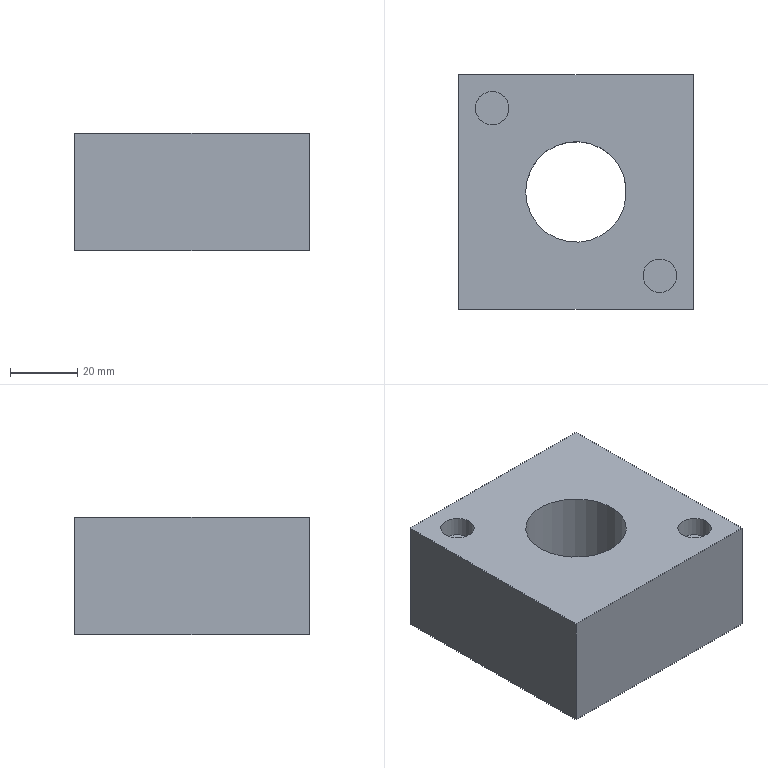Part | NX | features solid 2 | 1 solid | 11 faces | box 70 x 70 x 35 mm | volume 145817 mm3 | plane 8 | cylinder 3 | commonest cylinder face diameters 10 x2 30 x1
STEP:
#1=CARTESIAN_POINT('',(50.,-415.,-175.));
#2=VERTEX_POINT('',#1);
#3=CARTESIAN_POINT('',(55.,-415.,-175.));
#4=DIRECTION('',(0.,0.,-1.));
#5=DIRECTION('',(-1.,0.,0.));
#6=AXIS2_PLACEMENT_3D('',#3,#4,#5);
#7=CIRCLE('',#6,5.);
#8=EDGE_CURVE('',#2,#2,#7,.F.);
#9=ORIENTED_EDGE('',*,*,#8,.F.);
#10=EDGE_LOOP('',(#9));
#11=FACE_BOUND('',#10,.T.);
#12=CARTESIAN_POINT('',(65.,-440.,-175.));
#13=VERTEX_POINT('',#12);
#14=CARTESIAN_POINT('',(80.,-440.,-175.));
#15=DIRECTION('',(0.,0.,-1.));
#16=DIRECTION('',(-1.,0.,0.));
#17=AXIS2_PLACEMENT_3D('',#14,#15,#16);
#18=CIRCLE('',#17,15.);
#19=EDGE_CURVE('',#13,#13,#18,.T.);
#20=ORIENTED_EDGE('',*,*,#19,.T.);
#21=EDGE_LOOP('',(#20));
#22=FACE_BOUND('',#21,.T.);
#23=CARTESIAN_POINT('',(45.,-475.,-175.));
#24=VERTEX_POINT('',#23);
#25=CARTESIAN_POINT('',(45.,-405.,-175.));
#26=VERTEX_POINT('',#25);
#27=CARTESIAN_POINT('',(45.,-475.,-175.));
#28=DIRECTION('',(0.,1.,0.));
#29=VECTOR('',#28,1000.);
#30=LINE('',#27,#29);
#31=EDGE_CURVE('',#24,#26,#30,.T.);
#32=ORIENTED_EDGE('',*,*,#31,.F.);
#33=CARTESIAN_POINT('',(115.,-475.,-175.));
#34=VERTEX_POINT('',#33);
#35=CARTESIAN_POINT('',(115.,-475.,-175.));
#36=DIRECTION('',(-1.,0.,0.));
#37=VECTOR('',#36,1000.);
#38=LINE('',#35,#37);
#39=EDGE_CURVE('',#34,#24,#38,.T.);
#40=ORIENTED_EDGE('',*,*,#39,.F.);
#41=CARTESIAN_POINT('',(115.,-405.,-175.));
#42=VERTEX_POINT('',#41);
#43=CARTESIAN_POINT('',(115.,-405.,-175.));
#44=DIRECTION('',(0.,-1.,0.));
#45=VECTOR('',#44,1000.);
#46=LINE('',#43,#45);
#47=EDGE_CURVE('',#42,#34,#46,.T.);
#48=ORIENTED_EDGE('',*,*,#47,.F.);
#49=CARTESIAN_POINT('',(45.,-405.,-175.));
#50=DIRECTION('',(1.,0.,0.));
#51=VECTOR('',#50,1000.);
#52=LINE('',#49,#51);
#53=EDGE_CURVE('',#26,#42,#52,.T.);
#54=ORIENTED_EDGE('',*,*,#53,.F.);
#55=EDGE_LOOP('',(#32,#40,#48,#54));
#56=FACE_BOUND('',#55,.T.);
#57=CARTESIAN_POINT('',(100.,-465.,-175.));
#58=VERTEX_POINT('',#57);
#59=CARTESIAN_POINT('',(105.,-465.,-175.));
#60=DIRECTION('',(0.,0.,-1.));
#61=DIRECTION('',(-1.,0.,0.));
#62=AXIS2_PLACEMENT_3D('',#59,#60,#61);
#63=CIRCLE('',#62,5.);
#64=EDGE_CURVE('',#58,#58,#63,.F.);
#65=ORIENTED_EDGE('',*,*,#64,.F.);
#66=EDGE_LOOP('',(#65));
#67=FACE_BOUND('',#66,.T.);
#68=CARTESIAN_POINT('',(45.,-405.,-175.));
#69=DIRECTION('',(0.,0.,1.));
#70=DIRECTION('',(-1.,0.,0.));
#71=AXIS2_PLACEMENT_3D('',#68,#69,#70);
#72=PLANE('',#71);
#73=ADVANCED_FACE('',(#11,#22,#56,#67),#72,.T.);
#74=CARTESIAN_POINT('',(45.,-475.,-210.));
#75=VERTEX_POINT('',#74);
#76=CARTESIAN_POINT('',(45.,-405.,-210.));
#77=VERTEX_POINT('',#76);
#78=CARTESIAN_POINT('',(45.,-475.,-210.));
#79=DIRECTION('',(0.,1.,0.));
#80=VECTOR('',#79,1000.);
#81=LINE('',#78,#80);
#82=EDGE_CURVE('',#75,#77,#81,.T.);
#83=ORIENTED_EDGE('',*,*,#82,.F.);
#84=CARTESIAN_POINT('',(45.,-475.,-175.));
#85=DIRECTION('',(0.,0.,-1.));
#86=VECTOR('',#85,1000.);
#87=LINE('',#84,#86);
#88=EDGE_CURVE('',#24,#75,#87,.T.);
#89=ORIENTED_EDGE('',*,*,#88,.F.);
#90=ORIENTED_EDGE('',*,*,#31,.T.);
#91=CARTESIAN_POINT('',(45.,-405.,-175.));
#92=DIRECTION('',(0.,0.,-1.));
#93=VECTOR('',#92,1000.);
#94=LINE('',#91,#93);
#95=EDGE_CURVE('',#26,#77,#94,.T.);
#96=ORIENTED_EDGE('',*,*,#95,.T.);
#97=EDGE_LOOP('',(#83,#89,#90,#96));
#98=FACE_BOUND('',#97,.T.);
#99=CARTESIAN_POINT('',(45.,-475.,-175.));
#100=DIRECTION('',(1.,0.,0.));
#101=DIRECTION('',(0.,1.,0.));
#102=AXIS2_PLACEMENT_3D('',#99,#100,#101);
#103=PLANE('',#102);
#104=ADVANCED_FACE('',(#98),#103,.F.);
#105=CARTESIAN_POINT('',(115.,-405.,-210.));
#106=VERTEX_POINT('',#105);
#107=CARTESIAN_POINT('',(45.,-405.,-210.));
#108=DIRECTION('',(1.,0.,0.));
#109=VECTOR('',#108,1000.);
#110=LINE('',#107,#109);
#111=EDGE_CURVE('',#77,#106,#110,.T.);
#112=ORIENTED_EDGE('',*,*,#111,.F.);
#113=ORIENTED_EDGE('',*,*,#95,.F.);
#114=ORIENTED_EDGE('',*,*,#53,.T.);
#115=CARTESIAN_POINT('',(115.,-405.,-175.));
#116=DIRECTION('',(0.,0.,-1.));
#117=VECTOR('',#116,1000.);
#118=LINE('',#115,#117);
#119=EDGE_CURVE('',#42,#106,#118,.T.);
#120=ORIENTED_EDGE('',*,*,#119,.T.);
#121=EDGE_LOOP('',(#112,#113,#114,#120));
#122=FACE_BOUND('',#121,.T.);
#123=CARTESIAN_POINT('',(45.,-405.,-175.));
#124=DIRECTION('',(0.,-1.,0.));
#125=DIRECTION('',(0.,0.,1.));
#126=AXIS2_PLACEMENT_3D('',#123,#124,#125);
#127=PLANE('',#126);
#128=ADVANCED_FACE('',(#122),#127,.F.);
#129=CARTESIAN_POINT('',(115.,-475.,-210.));
#130=VERTEX_POINT('',#129);
#131=CARTESIAN_POINT('',(115.,-405.,-210.));
#132=DIRECTION('',(0.,-1.,0.));
#133=VECTOR('',#132,1000.);
#134=LINE('',#131,#133);
#135=EDGE_CURVE('',#106,#130,#134,.T.);
#136=ORIENTED_EDGE('',*,*,#135,.F.);
#137=ORIENTED_EDGE('',*,*,#119,.F.);
#138=ORIENTED_EDGE('',*,*,#47,.T.);
#139=CARTESIAN_POINT('',(115.,-475.,-175.));
#140=DIRECTION('',(0.,0.,-1.));
#141=VECTOR('',#140,1000.);
#142=LINE('',#139,#141);
#143=EDGE_CURVE('',#34,#130,#142,.T.);
#144=ORIENTED_EDGE('',*,*,#143,.T.);
#145=EDGE_LOOP('',(#136,#137,#138,#144));
#146=FACE_BOUND('',#145,.T.);
#147=CARTESIAN_POINT('',(115.,-405.,-175.));
#148=DIRECTION('',(-1.,0.,0.));
#149=DIRECTION('',(0.,0.,-1.));
#150=AXIS2_PLACEMENT_3D('',#147,#148,#149);
#151=PLANE('',#150);
#152=ADVANCED_FACE('',(#146),#151,.F.);
#153=ORIENTED_EDGE('',*,*,#19,.F.);
#154=EDGE_LOOP('',(#153));
#155=FACE_BOUND('',#154,.T.);
#156=CARTESIAN_POINT('',(65.,-440.,-210.));
#157=VERTEX_POINT('',#156);
#158=CARTESIAN_POINT('',(80.,-440.,-210.));
#159=DIRECTION('',(0.,0.,-1.));
#160=DIRECTION('',(-1.,0.,0.));
#161=AXIS2_PLACEMENT_3D('',#158,#159,#160);
#162=CIRCLE('',#161,15.);
#163=EDGE_CURVE('',#157,#157,#162,.T.);
#164=ORIENTED_EDGE('',*,*,#163,.T.);
#165=EDGE_LOOP('',(#164));
#166=FACE_BOUND('',#165,.T.);
#167=CARTESIAN_POINT('',(80.,-440.,-175.));
#168=DIRECTION('',(0.,0.,-1.));
#169=DIRECTION('',(1.,0.,0.));
#170=AXIS2_PLACEMENT_3D('',#167,#168,#169);
#171=CYLINDRICAL_SURFACE('',#170,15.);
#172=ADVANCED_FACE('',(#155,#166),#171,.F.);
#173=CARTESIAN_POINT('',(115.,-475.,-210.));
#174=DIRECTION('',(-1.,0.,0.));
#175=VECTOR('',#174,1000.);
#176=LINE('',#173,#175);
#177=EDGE_CURVE('',#130,#75,#176,.T.);
#178=ORIENTED_EDGE('',*,*,#177,.F.);
#179=ORIENTED_EDGE('',*,*,#143,.F.);
#180=ORIENTED_EDGE('',*,*,#39,.T.);
#181=ORIENTED_EDGE('',*,*,#88,.T.);
#182=EDGE_LOOP('',(#178,#179,#180,#181));
#183=FACE_BOUND('',#182,.T.);
#184=CARTESIAN_POINT('',(115.,-475.,-175.));
#185=DIRECTION('',(0.,1.,0.));
#186=DIRECTION('',(-1.,0.,0.));
#187=AXIS2_PLACEMENT_3D('',#184,#185,#186);
#188=PLANE('',#187);
#189=ADVANCED_FACE('',(#183),#188,.F.);
#190=ORIENTED_EDGE('',*,*,#163,.F.);
#191=EDGE_LOOP('',(#190));
#192=FACE_BOUND('',#191,.T.);
#193=ORIENTED_EDGE('',*,*,#82,.T.);
#194=ORIENTED_EDGE('',*,*,#111,.T.);
#195=ORIENTED_EDGE('',*,*,#135,.T.);
#196=ORIENTED_EDGE('',*,*,#177,.T.);
#197=EDGE_LOOP('',(#193,#194,#195,#196));
#198=FACE_BOUND('',#197,.T.);
#199=CARTESIAN_POINT('',(45.,-405.,-210.));
#200=DIRECTION('',(0.,0.,1.));
#201=DIRECTION('',(-1.,0.,0.));
#202=AXIS2_PLACEMENT_3D('',#199,#200,#201);
#203=PLANE('',#202);
#204=ADVANCED_FACE('',(#192,#198),#203,.F.);
#205=ORIENTED_EDGE('',*,*,#8,.T.);
#206=EDGE_LOOP('',(#205));
#207=FACE_BOUND('',#206,.T.);
#208=CARTESIAN_POINT('',(50.,-415.,-181.));
#209=VERTEX_POINT('',#208);
#210=CARTESIAN_POINT('',(55.,-415.,-181.));
#211=DIRECTION('',(0.,0.,-1.));
#212=DIRECTION('',(-1.,0.,0.));
#213=AXIS2_PLACEMENT_3D('',#210,#211,#212);
#214=CIRCLE('',#213,5.);
#215=EDGE_CURVE('',#209,#209,#214,.T.);
#216=ORIENTED_EDGE('',*,*,#215,.T.);
#217=EDGE_LOOP('',(#216));
#218=FACE_BOUND('',#217,.T.);
#219=CARTESIAN_POINT('',(55.,-415.,-171.));
#220=DIRECTION('',(0.,0.,-1.));
#221=DIRECTION('',(1.,0.,0.));
#222=AXIS2_PLACEMENT_3D('',#219,#220,#221);
#223=CYLINDRICAL_SURFACE('',#222,5.);
#224=ADVANCED_FACE('',(#207,#218),#223,.F.);
#225=ORIENTED_EDGE('',*,*,#215,.F.);
#226=EDGE_LOOP('',(#225));
#227=FACE_BOUND('',#226,.T.);
#228=CARTESIAN_POINT('',(55.,-415.,-181.));
#229=DIRECTION('',(0.,0.,1.));
#230=DIRECTION('',(-1.,0.,0.));
#231=AXIS2_PLACEMENT_3D('',#228,#229,#230);
#232=PLANE('',#231);
#233=ADVANCED_FACE('',(#227),#232,.T.);
#234=ORIENTED_EDGE('',*,*,#64,.T.);
#235=EDGE_LOOP('',(#234));
#236=FACE_BOUND('',#235,.T.);
#237=CARTESIAN_POINT('',(100.,-465.,-181.));
#238=VERTEX_POINT('',#237);
#239=CARTESIAN_POINT('',(105.,-465.,-181.));
#240=DIRECTION('',(0.,0.,-1.));
#241=DIRECTION('',(-1.,0.,0.));
#242=AXIS2_PLACEMENT_3D('',#239,#240,#241);
#243=CIRCLE('',#242,5.);
#244=EDGE_CURVE('',#238,#238,#243,.T.);
#245=ORIENTED_EDGE('',*,*,#244,.T.);
#246=EDGE_LOOP('',(#245));
#247=FACE_BOUND('',#246,.T.);
#248=CARTESIAN_POINT('',(105.,-465.,-171.));
#249=DIRECTION('',(0.,0.,-1.));
#250=DIRECTION('',(1.,0.,0.));
#251=AXIS2_PLACEMENT_3D('',#248,#249,#250);
#252=CYLINDRICAL_SURFACE('',#251,5.);
#253=ADVANCED_FACE('',(#236,#247),#252,.F.);
#254=ORIENTED_EDGE('',*,*,#244,.F.);
#255=EDGE_LOOP('',(#254));
#256=FACE_BOUND('',#255,.T.);
#257=CARTESIAN_POINT('',(105.,-465.,-181.));
#258=DIRECTION('',(0.,0.,1.));
#259=DIRECTION('',(-1.,0.,0.));
#260=AXIS2_PLACEMENT_3D('',#257,#258,#259);
#261=PLANE('',#260);
#262=ADVANCED_FACE('',(#256),#261,.T.);
#263=CLOSED_SHELL('',(#73,#104,#128,#152,#172,#189,#204,#224,#233,#253,#262));
#264=MANIFOLD_SOLID_BREP('',#263);
#265=(LENGTH_UNIT()NAMED_UNIT(*)SI_UNIT(.MILLI.,.METRE.));
#266=UNCERTAINTY_MEASURE_WITH_UNIT(LENGTH_MEASURE(0.00001),#265,'','');
#267=(NAMED_UNIT(*)PLANE_ANGLE_UNIT()SI_UNIT($,.RADIAN.));
#268=(NAMED_UNIT(*)SI_UNIT($,.STERADIAN.)SOLID_ANGLE_UNIT());
#269=(GEOMETRIC_REPRESENTATION_CONTEXT(3)GLOBAL_UNCERTAINTY_ASSIGNED_CONTEXT((#266))GLOBAL_UNIT_ASSIGNED_CONTEXT((#265,#267,#268))REPRESENTATION_CONTEXT('',''));
#270=ADVANCED_BREP_SHAPE_REPRESENTATION('',(#264),#269);